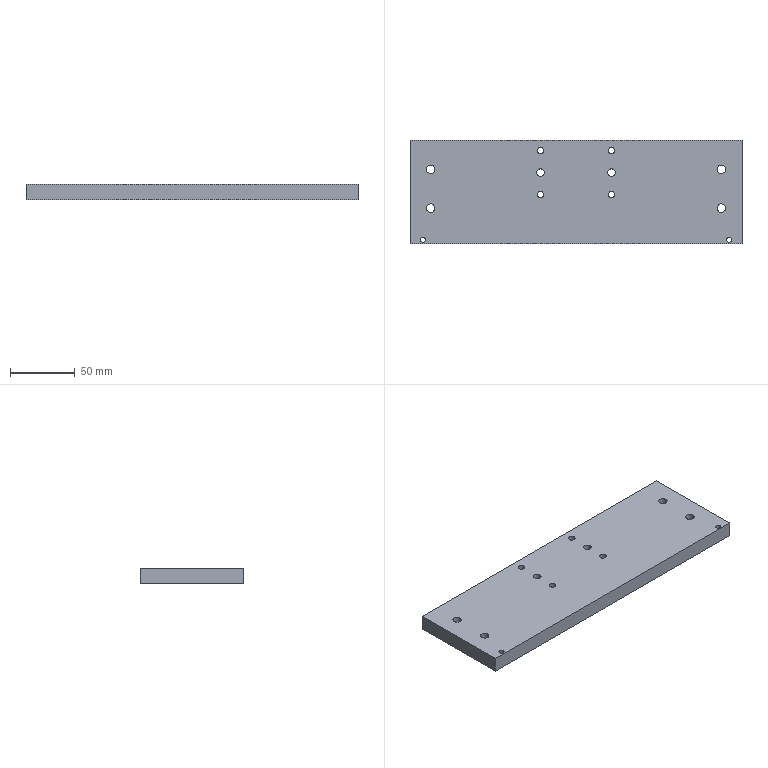Part | STEP file | E01 | 1 solid | 42 faces | box 257 x 80 x 12 mm | volume 241598 mm3 | cylinder 32 | plane 10 | commonest cylinder face diameters 5 x8 6.6 x8 11 x8 4 x4 6 x4